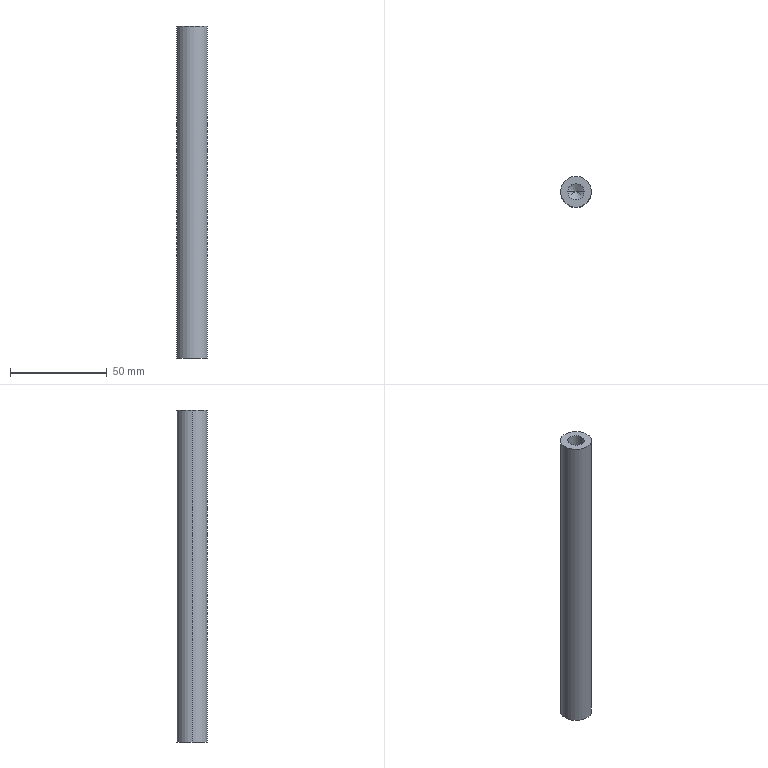Part | STEP file | B1-019 | 1 solid | 12 faces | box 16 x 16 x 172 mm | volume 32897 mm3 | cylinder 6 | cone 4 | plane 2 | commonest cylinder face diameters 8.5 x4 16 x2
STEP:
#1=CARTESIAN_POINT('',(0.,0.,0.));
#2=DIRECTION('',(0.,0.,1.));
#3=DIRECTION('',(1.,0.,0.));
#4=AXIS2_PLACEMENT_3D('',#1,#2,#3);
#5=CARTESIAN_POINT('',(4.25,0.,72.));
#6=VERTEX_POINT('',#5);
#7=CARTESIAN_POINT('',(4.25,0.,86.));
#8=VERTEX_POINT('',#7);
#9=CARTESIAN_POINT('',(4.25,0.,86.));
#10=DIRECTION('',(0.,0.,1.));
#11=VECTOR('',#10,1.);
#12=LINE('',#9,#11);
#13=CARTESIAN_POINT('',(0.,0.,86.));
#14=DIRECTION('',(0.,0.,1.));
#15=DIRECTION('',(1.,0.,0.));
#16=AXIS2_PLACEMENT_3D('',#13,#14,#15);
#17=CYLINDRICAL_SURFACE('',#16,4.25);
#18=CARTESIAN_POINT('',(6.283,0.));
#19=DIRECTION('',(0.,1.));
#20=VECTOR('',#19,1.);
#21=LINE('',#18,#20);
#22=(GEOMETRIC_REPRESENTATION_CONTEXT(2)PARAMETRIC_REPRESENTATION_CONTEXT()REPRESENTATION_CONTEXT('',''));
#23=DEFINITIONAL_REPRESENTATION('',(#21),#22);
#24=PCURVE('',#17,#23);
#25=CARTESIAN_POINT('',(0.,0.,86.));
#26=DIRECTION('',(0.,0.,1.));
#27=DIRECTION('',(1.,0.,0.));
#28=AXIS2_PLACEMENT_3D('',#25,#26,#27);
#29=CYLINDRICAL_SURFACE('',#28,4.25);
#30=CARTESIAN_POINT('',(0.,0.));
#31=DIRECTION('',(0.,1.));
#32=VECTOR('',#31,1.);
#33=LINE('',#30,#32);
#34=(GEOMETRIC_REPRESENTATION_CONTEXT(2)PARAMETRIC_REPRESENTATION_CONTEXT()REPRESENTATION_CONTEXT('',''));
#35=DEFINITIONAL_REPRESENTATION('',(#33),#34);
#36=PCURVE('',#29,#35);
#37=SURFACE_CURVE('',#12,(#24,#36),.PCURVE_S1.);
#38=EDGE_CURVE('',#6,#8,#37,.T.);
#39=ORIENTED_EDGE('',*,*,#38,.T.);
#40=CARTESIAN_POINT('',(-4.25,0.,86.));
#41=VERTEX_POINT('',#40);
#42=CARTESIAN_POINT('',(0.,0.,86.));
#43=DIRECTION('',(0.,0.,1.));
#44=DIRECTION('',(1.,0.,0.));
#45=AXIS2_PLACEMENT_3D('',#42,#43,#44);
#46=CIRCLE('',#45,4.25);
#47=CARTESIAN_POINT('',(0.,0.));
#48=DIRECTION('',(1.,0.));
#49=VECTOR('',#48,1.);
#50=LINE('',#47,#49);
#51=(GEOMETRIC_REPRESENTATION_CONTEXT(2)PARAMETRIC_REPRESENTATION_CONTEXT()REPRESENTATION_CONTEXT('',''));
#52=DEFINITIONAL_REPRESENTATION('',(#50),#51);
#53=PCURVE('',#17,#52);
#54=CARTESIAN_POINT('',(0.,0.,86.));
#55=DIRECTION('',(0.,0.,1.));
#56=DIRECTION('',(1.,0.,0.));
#57=AXIS2_PLACEMENT_3D('',#54,#55,#56);
#58=PLANE('',#57);
#59=CARTESIAN_POINT('',(0.,0.));
#60=DIRECTION('',(1.,0.));
#61=AXIS2_PLACEMENT_2D('',#59,#60);
#62=CIRCLE('',#61,4.25);
#63=(GEOMETRIC_REPRESENTATION_CONTEXT(2)PARAMETRIC_REPRESENTATION_CONTEXT()REPRESENTATION_CONTEXT('',''));
#64=DEFINITIONAL_REPRESENTATION('',(#62),#63);
#65=PCURVE('',#58,#64);
#66=SURFACE_CURVE('',#46,(#53,#65),.PCURVE_S1.);
#67=EDGE_CURVE('',#41,#8,#66,.T.);
#68=ORIENTED_EDGE('',*,*,#67,.F.);
#69=CARTESIAN_POINT('',(-4.25,0.,72.));
#70=VERTEX_POINT('',#69);
#71=CARTESIAN_POINT('',(-4.25,0.,86.));
#72=DIRECTION('',(0.,0.,1.));
#73=VECTOR('',#72,1.);
#74=LINE('',#71,#73);
#75=CARTESIAN_POINT('',(3.142,0.));
#76=DIRECTION('',(0.,1.));
#77=VECTOR('',#76,1.);
#78=LINE('',#75,#77);
#79=(GEOMETRIC_REPRESENTATION_CONTEXT(2)PARAMETRIC_REPRESENTATION_CONTEXT()REPRESENTATION_CONTEXT('',''));
#80=DEFINITIONAL_REPRESENTATION('',(#78),#79);
#81=PCURVE('',#17,#80);
#82=CARTESIAN_POINT('',(3.142,0.));
#83=DIRECTION('',(0.,1.));
#84=VECTOR('',#83,1.);
#85=LINE('',#82,#84);
#86=(GEOMETRIC_REPRESENTATION_CONTEXT(2)PARAMETRIC_REPRESENTATION_CONTEXT()REPRESENTATION_CONTEXT('',''));
#87=DEFINITIONAL_REPRESENTATION('',(#85),#86);
#88=PCURVE('',#29,#87);
#89=SURFACE_CURVE('',#74,(#81,#88),.PCURVE_S1.);
#90=EDGE_CURVE('',#70,#41,#89,.T.);
#91=ORIENTED_EDGE('',*,*,#90,.F.);
#92=CARTESIAN_POINT('',(0.,0.,72.));
#93=DIRECTION('',(0.,0.,1.));
#94=DIRECTION('',(1.,0.,0.));
#95=AXIS2_PLACEMENT_3D('',#92,#93,#94);
#96=CIRCLE('',#95,4.25);
#97=CARTESIAN_POINT('',(0.,-14.));
#98=DIRECTION('',(1.,0.));
#99=VECTOR('',#98,1.);
#100=LINE('',#97,#99);
#101=(GEOMETRIC_REPRESENTATION_CONTEXT(2)PARAMETRIC_REPRESENTATION_CONTEXT()REPRESENTATION_CONTEXT('',''));
#102=DEFINITIONAL_REPRESENTATION('',(#100),#101);
#103=PCURVE('',#17,#102);
#104=CARTESIAN_POINT('',(0.,0.,72.));
#105=DIRECTION('',(0.,0.,1.));
#106=DIRECTION('',(1.,0.,0.));
#107=AXIS2_PLACEMENT_3D('',#104,#105,#106);
#108=CONICAL_SURFACE('',#107,4.25,1.03);
#109=CARTESIAN_POINT('',(0.,0.));
#110=DIRECTION('',(1.,0.));
#111=VECTOR('',#110,1.);
#112=LINE('',#109,#111);
#113=(GEOMETRIC_REPRESENTATION_CONTEXT(2)PARAMETRIC_REPRESENTATION_CONTEXT()REPRESENTATION_CONTEXT('',''));
#114=DEFINITIONAL_REPRESENTATION('',(#112),#113);
#115=PCURVE('',#108,#114);
#116=SURFACE_CURVE('',#96,(#103,#115),.PCURVE_S1.);
#117=EDGE_CURVE('',#70,#6,#116,.T.);
#118=ORIENTED_EDGE('',*,*,#117,.T.);
#119=EDGE_LOOP('',(#39,#68,#91,#118));
#120=FACE_BOUND('',#119,.F.);
#121=ADVANCED_FACE('',(#120),#17,.F.);
#122=ORIENTED_EDGE('',*,*,#117,.F.);
#123=CARTESIAN_POINT('',(0.,0.,69.446));
#124=VERTEX_POINT('',#123);
#125=CARTESIAN_POINT('',(-4.25,0.,72.));
#126=DIRECTION('',(-0.8572,0.,0.515));
#127=VECTOR('',#126,1.);
#128=LINE('',#125,#127);
#129=CARTESIAN_POINT('',(3.142,0.));
#130=DIRECTION('',(0.,1.));
#131=VECTOR('',#130,1.);
#132=LINE('',#129,#131);
#133=(GEOMETRIC_REPRESENTATION_CONTEXT(2)PARAMETRIC_REPRESENTATION_CONTEXT()REPRESENTATION_CONTEXT('',''));
#134=DEFINITIONAL_REPRESENTATION('',(#132),#133);
#135=PCURVE('',#108,#134);
#136=CARTESIAN_POINT('',(0.,0.,72.));
#137=DIRECTION('',(0.,0.,1.));
#138=DIRECTION('',(1.,0.,0.));
#139=AXIS2_PLACEMENT_3D('',#136,#137,#138);
#140=CONICAL_SURFACE('',#139,4.25,1.03);
#141=CARTESIAN_POINT('',(3.142,0.));
#142=DIRECTION('',(0.,1.));
#143=VECTOR('',#142,1.);
#144=LINE('',#141,#143);
#145=(GEOMETRIC_REPRESENTATION_CONTEXT(2)PARAMETRIC_REPRESENTATION_CONTEXT()REPRESENTATION_CONTEXT('',''));
#146=DEFINITIONAL_REPRESENTATION('',(#144),#145);
#147=PCURVE('',#140,#146);
#148=SURFACE_CURVE('',#128,(#135,#147),.PCURVE_S1.);
#149=EDGE_CURVE('',#124,#70,#148,.T.);
#150=ORIENTED_EDGE('',*,*,#149,.F.);
#151=CARTESIAN_POINT('',(4.25,0.,72.));
#152=DIRECTION('',(0.8572,0.,0.515));
#153=VECTOR('',#152,1.);
#154=LINE('',#151,#153);
#155=CARTESIAN_POINT('',(6.283,-2.554));
#156=CARTESIAN_POINT('',(6.283,-2.515));
#157=CARTESIAN_POINT('',(6.283,-2.438));
#158=CARTESIAN_POINT('',(6.283,-2.322));
#159=CARTESIAN_POINT('',(6.283,-2.205));
#160=CARTESIAN_POINT('',(6.283,-2.089));
#161=CARTESIAN_POINT('',(6.283,-1.973));
#162=CARTESIAN_POINT('',(6.283,-1.857));
#163=CARTESIAN_POINT('',(6.283,-1.741));
#164=CARTESIAN_POINT('',(6.283,-1.625));
#165=CARTESIAN_POINT('',(6.283,-1.509));
#166=CARTESIAN_POINT('',(6.283,-1.393));
#167=CARTESIAN_POINT('',(6.283,-1.277));
#168=CARTESIAN_POINT('',(6.283,-1.161));
#169=CARTESIAN_POINT('',(6.283,-1.045));
#170=CARTESIAN_POINT('',(6.283,-0.9286));
#171=CARTESIAN_POINT('',(6.283,-0.8125));
#172=CARTESIAN_POINT('',(6.283,-0.6965));
#173=CARTESIAN_POINT('',(6.283,-0.5804));
#174=CARTESIAN_POINT('',(6.283,-0.4643));
#175=CARTESIAN_POINT('',(6.283,-0.3482));
#176=CARTESIAN_POINT('',(6.283,-0.2322));
#177=CARTESIAN_POINT('',(6.283,-0.1161));
#178=CARTESIAN_POINT('',(6.283,-0.03869));
#179=CARTESIAN_POINT('',(6.283,0.));
#180=B_SPLINE_CURVE_WITH_KNOTS('',3,(#155,#156,#157,#158,#159,#160,#161,#162,#163,#164,#165,#166,#167,#168,#169,#170,#171,#172,#173,#174,#175,#176,#177,#178,#179),.UNSPECIFIED.,.F.,.F.,(4,1,1,1,1,1,1,1,1,1,1,1,1,1,1,1,1,1,1,1,1,1,4),(-4.958,-4.733,-4.507,-4.282,-4.057,-3.831,-3.606,-3.381,-3.155,-2.93,-2.704,-2.479,-2.254,-2.028,-1.803,-1.578,-1.352,-1.127,-0.9015,-0.6761,-0.4507,-0.2254,0.),.QUASI_UNIFORM_KNOTS.);
#181=(GEOMETRIC_REPRESENTATION_CONTEXT(2)PARAMETRIC_REPRESENTATION_CONTEXT()REPRESENTATION_CONTEXT('',''));
#182=DEFINITIONAL_REPRESENTATION('',(#180),#181);
#183=PCURVE('',#108,#182);
#184=CARTESIAN_POINT('',(0.,-2.554));
#185=CARTESIAN_POINT('',(0.,-2.515));
#186=CARTESIAN_POINT('',(0.,-2.438));
#187=CARTESIAN_POINT('',(0.,-2.322));
#188=CARTESIAN_POINT('',(0.,-2.205));
#189=CARTESIAN_POINT('',(0.,-2.089));
#190=CARTESIAN_POINT('',(0.,-1.973));
#191=CARTESIAN_POINT('',(0.,-1.857));
#192=CARTESIAN_POINT('',(0.,-1.741));
#193=CARTESIAN_POINT('',(0.,-1.625));
#194=CARTESIAN_POINT('',(0.,-1.509));
#195=CARTESIAN_POINT('',(0.,-1.393));
#196=CARTESIAN_POINT('',(0.,-1.277));
#197=CARTESIAN_POINT('',(0.,-1.161));
#198=CARTESIAN_POINT('',(0.,-1.045));
#199=CARTESIAN_POINT('',(0.,-0.9286));
#200=CARTESIAN_POINT('',(0.,-0.8125));
#201=CARTESIAN_POINT('',(0.,-0.6965));
#202=CARTESIAN_POINT('',(0.,-0.5804));
#203=CARTESIAN_POINT('',(0.,-0.4643));
#204=CARTESIAN_POINT('',(0.,-0.3482));
#205=CARTESIAN_POINT('',(0.,-0.2322));
#206=CARTESIAN_POINT('',(0.,-0.1161));
#207=CARTESIAN_POINT('',(0.,-0.03869));
#208=CARTESIAN_POINT('',(0.,0.));
#209=B_SPLINE_CURVE_WITH_KNOTS('',3,(#184,#185,#186,#187,#188,#189,#190,#191,#192,#193,#194,#195,#196,#197,#198,#199,#200,#201,#202,#203,#204,#205,#206,#207,#208),.UNSPECIFIED.,.F.,.F.,(4,1,1,1,1,1,1,1,1,1,1,1,1,1,1,1,1,1,1,1,1,1,4),(-4.958,-4.733,-4.507,-4.282,-4.057,-3.831,-3.606,-3.381,-3.155,-2.93,-2.704,-2.479,-2.254,-2.028,-1.803,-1.578,-1.352,-1.127,-0.9015,-0.6761,-0.4507,-0.2254,0.),.QUASI_UNIFORM_KNOTS.);
#210=(GEOMETRIC_REPRESENTATION_CONTEXT(2)PARAMETRIC_REPRESENTATION_CONTEXT()REPRESENTATION_CONTEXT('',''));
#211=DEFINITIONAL_REPRESENTATION('',(#209),#210);
#212=PCURVE('',#140,#211);
#213=SURFACE_CURVE('',#154,(#183,#212),.PCURVE_S1.);
#214=EDGE_CURVE('',#124,#6,#213,.T.);
#215=ORIENTED_EDGE('',*,*,#214,.T.);
#216=EDGE_LOOP('',(#122,#150,#215));
#217=FACE_BOUND('',#216,.F.);
#218=ADVANCED_FACE('',(#217),#108,.F.);
#219=CARTESIAN_POINT('',(-4.25,0.,-72.));
#220=VERTEX_POINT('',#219);
#221=CARTESIAN_POINT('',(-4.25,0.,-86.));
#222=VERTEX_POINT('',#221);
#223=CARTESIAN_POINT('',(-4.25,0.,-86.));
#224=DIRECTION('',(0.,0.,-1.));
#225=VECTOR('',#224,1.);
#226=LINE('',#223,#225);
#227=CARTESIAN_POINT('',(0.,0.,-86.));
#228=DIRECTION('',(0.,0.,-1.));
#229=DIRECTION('',(-1.,0.,0.));
#230=AXIS2_PLACEMENT_3D('',#227,#228,#229);
#231=CYLINDRICAL_SURFACE('',#230,4.25);
#232=CARTESIAN_POINT('',(6.283,0.));
#233=DIRECTION('',(0.,1.));
#234=VECTOR('',#233,1.);
#235=LINE('',#232,#234);
#236=(GEOMETRIC_REPRESENTATION_CONTEXT(2)PARAMETRIC_REPRESENTATION_CONTEXT()REPRESENTATION_CONTEXT('',''));
#237=DEFINITIONAL_REPRESENTATION('',(#235),#236);
#238=PCURVE('',#231,#237);
#239=CARTESIAN_POINT('',(0.,0.,-86.));
#240=DIRECTION('',(0.,0.,-1.));
#241=DIRECTION('',(-1.,0.,0.));
#242=AXIS2_PLACEMENT_3D('',#239,#240,#241);
#243=CYLINDRICAL_SURFACE('',#242,4.25);
#244=CARTESIAN_POINT('',(0.,0.));
#245=DIRECTION('',(0.,1.));
#246=VECTOR('',#245,1.);
#247=LINE('',#244,#246);
#248=(GEOMETRIC_REPRESENTATION_CONTEXT(2)PARAMETRIC_REPRESENTATION_CONTEXT()REPRESENTATION_CONTEXT('',''));
#249=DEFINITIONAL_REPRESENTATION('',(#247),#248);
#250=PCURVE('',#243,#249);
#251=SURFACE_CURVE('',#226,(#238,#250),.PCURVE_S1.);
#252=EDGE_CURVE('',#220,#222,#251,.T.);
#253=ORIENTED_EDGE('',*,*,#252,.T.);
#254=CARTESIAN_POINT('',(4.25,0.,-86.));
#255=VERTEX_POINT('',#254);
#256=CARTESIAN_POINT('',(0.,0.,-86.));
#257=DIRECTION('',(0.,0.,-1.));
#258=DIRECTION('',(-1.,0.,0.));
#259=AXIS2_PLACEMENT_3D('',#256,#257,#258);
#260=CIRCLE('',#259,4.25);
#261=CARTESIAN_POINT('',(0.,0.));
#262=DIRECTION('',(1.,0.));
#263=VECTOR('',#262,1.);
#264=LINE('',#261,#263);
#265=(GEOMETRIC_REPRESENTATION_CONTEXT(2)PARAMETRIC_REPRESENTATION_CONTEXT()REPRESENTATION_CONTEXT('',''));
#266=DEFINITIONAL_REPRESENTATION('',(#264),#265);
#267=PCURVE('',#231,#266);
#268=CARTESIAN_POINT('',(0.,0.,-86.));
#269=DIRECTION('',(0.,0.,1.));
#270=DIRECTION('',(1.,0.,0.));
#271=AXIS2_PLACEMENT_3D('',#268,#269,#270);
#272=PLANE('',#271);
#273=CARTESIAN_POINT('',(-4.25,0.));
#274=CARTESIAN_POINT('',(-4.25,7.361));
#275=CARTESIAN_POINT('',(2.125,3.681));
#276=CARTESIAN_POINT('',(8.5,0.));
#277=CARTESIAN_POINT('',(2.125,-3.681));
#278=CARTESIAN_POINT('',(-4.25,-7.361));
#279=CARTESIAN_POINT('',(-4.25,0.));
#280=(BOUNDED_CURVE()B_SPLINE_CURVE(2,(#273,#274,#275,#276,#277,#278,#279),.UNSPECIFIED.,.T.,.F.)B_SPLINE_CURVE_WITH_KNOTS((1,2,2,2,2,1),(-2.094,0.,2.094,4.189,6.283,8.378),.UNSPECIFIED.)CURVE()GEOMETRIC_REPRESENTATION_ITEM()RATIONAL_B_SPLINE_CURVE((1.,0.5,1.,0.5,1.,0.5,1.))REPRESENTATION_ITEM(''));
#281=(GEOMETRIC_REPRESENTATION_CONTEXT(2)PARAMETRIC_REPRESENTATION_CONTEXT()REPRESENTATION_CONTEXT('',''));
#282=DEFINITIONAL_REPRESENTATION('',(#280),#281);
#283=PCURVE('',#272,#282);
#284=SURFACE_CURVE('',#260,(#267,#283),.PCURVE_S1.);
#285=EDGE_CURVE('',#255,#222,#284,.T.);
#286=ORIENTED_EDGE('',*,*,#285,.F.);
#287=CARTESIAN_POINT('',(4.25,0.,-72.));
#288=VERTEX_POINT('',#287);
#289=CARTESIAN_POINT('',(4.25,0.,-86.));
#290=DIRECTION('',(0.,0.,-1.));
#291=VECTOR('',#290,1.);
#292=LINE('',#289,#291);
#293=CARTESIAN_POINT('',(3.142,0.));
#294=DIRECTION('',(0.,1.));
#295=VECTOR('',#294,1.);
#296=LINE('',#293,#295);
#297=(GEOMETRIC_REPRESENTATION_CONTEXT(2)PARAMETRIC_REPRESENTATION_CONTEXT()REPRESENTATION_CONTEXT('',''));
#298=DEFINITIONAL_REPRESENTATION('',(#296),#297);
#299=PCURVE('',#231,#298);
#300=CARTESIAN_POINT('',(3.142,0.));
#301=DIRECTION('',(0.,1.));
#302=VECTOR('',#301,1.);
#303=LINE('',#300,#302);
#304=(GEOMETRIC_REPRESENTATION_CONTEXT(2)PARAMETRIC_REPRESENTATION_CONTEXT()REPRESENTATION_CONTEXT('',''));
#305=DEFINITIONAL_REPRESENTATION('',(#303),#304);
#306=PCURVE('',#243,#305);
#307=SURFACE_CURVE('',#292,(#299,#306),.PCURVE_S1.);
#308=EDGE_CURVE('',#288,#255,#307,.T.);
#309=ORIENTED_EDGE('',*,*,#308,.F.);
#310=CARTESIAN_POINT('',(0.,0.,-72.));
#311=DIRECTION('',(0.,0.,-1.));
#312=DIRECTION('',(-1.,0.,0.));
#313=AXIS2_PLACEMENT_3D('',#310,#311,#312);
#314=CIRCLE('',#313,4.25);
#315=CARTESIAN_POINT('',(0.,-14.));
#316=DIRECTION('',(1.,0.));
#317=VECTOR('',#316,1.);
#318=LINE('',#315,#317);
#319=(GEOMETRIC_REPRESENTATION_CONTEXT(2)PARAMETRIC_REPRESENTATION_CONTEXT()REPRESENTATION_CONTEXT('',''));
#320=DEFINITIONAL_REPRESENTATION('',(#318),#319);
#321=PCURVE('',#231,#320);
#322=CARTESIAN_POINT('',(0.,0.,-72.));
#323=DIRECTION('',(0.,0.,-1.));
#324=DIRECTION('',(-1.,0.,0.));
#325=AXIS2_PLACEMENT_3D('',#322,#323,#324);
#326=CONICAL_SURFACE('',#325,4.25,1.03);
#327=CARTESIAN_POINT('',(0.,0.));
#328=DIRECTION('',(1.,0.));
#329=VECTOR('',#328,1.);
#330=LINE('',#327,#329);
#331=(GEOMETRIC_REPRESENTATION_CONTEXT(2)PARAMETRIC_REPRESENTATION_CONTEXT()REPRESENTATION_CONTEXT('',''));
#332=DEFINITIONAL_REPRESENTATION('',(#330),#331);
#333=PCURVE('',#326,#332);
#334=SURFACE_CURVE('',#314,(#321,#333),.PCURVE_S1.);
#335=EDGE_CURVE('',#288,#220,#334,.T.);
#336=ORIENTED_EDGE('',*,*,#335,.T.);
#337=EDGE_LOOP('',(#253,#286,#309,#336));
#338=FACE_BOUND('',#337,.F.);
#339=ADVANCED_FACE('',(#338),#231,.F.);
#340=ORIENTED_EDGE('',*,*,#335,.F.);
#341=CARTESIAN_POINT('',(0.,0.,-69.446));
#342=VERTEX_POINT('',#341);
#343=CARTESIAN_POINT('',(4.25,0.,-72.));
#344=DIRECTION('',(0.8572,0.,-0.515));
#345=VECTOR('',#344,1.);
#346=LINE('',#343,#345);
#347=CARTESIAN_POINT('',(3.142,-2.554));
#348=CARTESIAN_POINT('',(3.142,-2.515));
#349=CARTESIAN_POINT('',(3.142,-2.438));
#350=CARTESIAN_POINT('',(3.142,-2.322));
#351=CARTESIAN_POINT('',(3.142,-2.205));
#352=CARTESIAN_POINT('',(3.142,-2.089));
#353=CARTESIAN_POINT('',(3.142,-1.973));
#354=CARTESIAN_POINT('',(3.142,-1.857));
#355=CARTESIAN_POINT('',(3.142,-1.741));
#356=CARTESIAN_POINT('',(3.142,-1.625));
#357=CARTESIAN_POINT('',(3.142,-1.509));
#358=CARTESIAN_POINT('',(3.142,-1.393));
#359=CARTESIAN_POINT('',(3.142,-1.277));
#360=CARTESIAN_POINT('',(3.142,-1.161));
#361=CARTESIAN_POINT('',(3.142,-1.045));
#362=CARTESIAN_POINT('',(3.142,-0.9286));
#363=CARTESIAN_POINT('',(3.142,-0.8125));
#364=CARTESIAN_POINT('',(3.142,-0.6965));
#365=CARTESIAN_POINT('',(3.142,-0.5804));
#366=CARTESIAN_POINT('',(3.142,-0.4643));
#367=CARTESIAN_POINT('',(3.142,-0.3482));
#368=CARTESIAN_POINT('',(3.142,-0.2322));
#369=CARTESIAN_POINT('',(3.142,-0.1161));
#370=CARTESIAN_POINT('',(3.142,-0.03869));
#371=CARTESIAN_POINT('',(3.142,0.));
#372=B_SPLINE_CURVE_WITH_KNOTS('',3,(#347,#348,#349,#350,#351,#352,#353,#354,#355,#356,#357,#358,#359,#360,#361,#362,#363,#364,#365,#366,#367,#368,#369,#370,#371),.UNSPECIFIED.,.F.,.F.,(4,1,1,1,1,1,1,1,1,1,1,1,1,1,1,1,1,1,1,1,1,1,4),(-4.958,-4.733,-4.507,-4.282,-4.057,-3.831,-3.606,-3.381,-3.155,-2.93,-2.704,-2.479,-2.254,-2.028,-1.803,-1.578,-1.352,-1.127,-0.9015,-0.6761,-0.4507,-0.2254,0.),.QUASI_UNIFORM_KNOTS.);
#373=(GEOMETRIC_REPRESENTATION_CONTEXT(2)PARAMETRIC_REPRESENTATION_CONTEXT()REPRESENTATION_CONTEXT('',''));
#374=DEFINITIONAL_REPRESENTATION('',(#372),#373);
#375=PCURVE('',#326,#374);
#376=CARTESIAN_POINT('',(0.,0.,-72.));
#377=DIRECTION('',(0.,0.,-1.));
#378=DIRECTION('',(-1.,0.,0.));
#379=AXIS2_PLACEMENT_3D('',#376,#377,#378);
#380=CONICAL_SURFACE('',#379,4.25,1.03);
#381=CARTESIAN_POINT('',(3.142,-2.554));
#382=CARTESIAN_POINT('',(3.142,-2.515));
#383=CARTESIAN_POINT('',(3.142,-2.438));
#384=CARTESIAN_POINT('',(3.142,-2.322));
#385=CARTESIAN_POINT('',(3.142,-2.205));
#386=CARTESIAN_POINT('',(3.142,-2.089));
#387=CARTESIAN_POINT('',(3.142,-1.973));
#388=CARTESIAN_POINT('',(3.142,-1.857));
#389=CARTESIAN_POINT('',(3.142,-1.741));
#390=CARTESIAN_POINT('',(3.142,-1.625));
#391=CARTESIAN_POINT('',(3.142,-1.509));
#392=CARTESIAN_POINT('',(3.142,-1.393));
#393=CARTESIAN_POINT('',(3.142,-1.277));
#394=CARTESIAN_POINT('',(3.142,-1.161));
#395=CARTESIAN_POINT('',(3.142,-1.045));
#396=CARTESIAN_POINT('',(3.142,-0.9286));
#397=CARTESIAN_POINT('',(3.142,-0.8125));
#398=CARTESIAN_POINT('',(3.142,-0.6965));
#399=CARTESIAN_POINT('',(3.142,-0.5804));
#400=CARTESIAN_POINT('',(3.142,-0.4643));
#401=CARTESIAN_POINT('',(3.142,-0.3482));
#402=CARTESIAN_POINT('',(3.142,-0.2322));
#403=CARTESIAN_POINT('',(3.142,-0.1161));
#404=CARTESIAN_POINT('',(3.142,-0.03869));
#405=CARTESIAN_POINT('',(3.142,0.));
#406=B_SPLINE_CURVE_WITH_KNOTS('',3,(#381,#382,#383,#384,#385,#386,#387,#388,#389,#390,#391,#392,#393,#394,#395,#396,#397,#398,#399,#400,#401,#402,#403,#404,#405),.UNSPECIFIED.,.F.,.F.,(4,1,1,1,1,1,1,1,1,1,1,1,1,1,1,1,1,1,1,1,1,1,4),(-4.958,-4.733,-4.507,-4.282,-4.057,-3.831,-3.606,-3.381,-3.155,-2.93,-2.704,-2.479,-2.254,-2.028,-1.803,-1.578,-1.352,-1.127,-0.9015,-0.6761,-0.4507,-0.2254,0.),.QUASI_UNIFORM_KNOTS.);
#407=(GEOMETRIC_REPRESENTATION_CONTEXT(2)PARAMETRIC_REPRESENTATION_CONTEXT()REPRESENTATION_CONTEXT('',''));
#408=DEFINITIONAL_REPRESENTATION('',(#406),#407);
#409=PCURVE('',#380,#408);
#410=SURFACE_CURVE('',#346,(#375,#409),.PCURVE_S1.);
#411=EDGE_CURVE('',#342,#288,#410,.T.);
#412=ORIENTED_EDGE('',*,*,#411,.F.);
#413=CARTESIAN_POINT('',(-4.25,0.,-72.));
#414=DIRECTION('',(-0.8572,0.,-0.515));
#415=VECTOR('',#414,1.);
#416=LINE('',#413,#415);
#417=CARTESIAN_POINT('',(6.283,0.));
#418=DIRECTION('',(0.,1.));
#419=VECTOR('',#418,1.);
#420=LINE('',#417,#419);
#421=(GEOMETRIC_REPRESENTATION_CONTEXT(2)PARAMETRIC_REPRESENTATION_CONTEXT()REPRESENTATION_CONTEXT('',''));
#422=DEFINITIONAL_REPRESENTATION('',(#420),#421);
#423=PCURVE('',#326,#422);
#424=CARTESIAN_POINT('',(0.,0.));
#425=DIRECTION('',(0.,1.));
#426=VECTOR('',#425,1.);
#427=LINE('',#424,#426);
#428=(GEOMETRIC_REPRESENTATION_CONTEXT(2)PARAMETRIC_REPRESENTATION_CONTEXT()REPRESENTATION_CONTEXT('',''));
#429=DEFINITIONAL_REPRESENTATION('',(#427),#428);
#430=PCURVE('',#380,#429);
#431=SURFACE_CURVE('',#416,(#423,#430),.PCURVE_S1.);
#432=EDGE_CURVE('',#342,#220,#431,.T.);
#433=ORIENTED_EDGE('',*,*,#432,.T.);
#434=EDGE_LOOP('',(#340,#412,#433));
#435=FACE_BOUND('',#434,.F.);
#436=ADVANCED_FACE('',(#435),#326,.F.);
#437=CARTESIAN_POINT('',(8.,0.,86.));
#438=VERTEX_POINT('',#437);
#439=CARTESIAN_POINT('',(-8.,0.,86.));
#440=VERTEX_POINT('',#439);
#441=CARTESIAN_POINT('',(0.,0.,86.));
#442=DIRECTION('',(0.,0.,1.));
#443=DIRECTION('',(1.,0.,0.));
#444=AXIS2_PLACEMENT_3D('',#441,#442,#443);
#445=CIRCLE('',#444,8.);
#446=CARTESIAN_POINT('',(0.,0.,86.));
#447=DIRECTION('',(0.,0.,-1.));
#448=DIRECTION('',(-1.,0.,0.));
#449=AXIS2_PLACEMENT_3D('',#446,#447,#448);
#450=CYLINDRICAL_SURFACE('',#449,8.);
#451=CARTESIAN_POINT('',(3.142,0.));
#452=DIRECTION('',(-1.,0.));
#453=VECTOR('',#452,1.);
#454=LINE('',#451,#453);
#455=(GEOMETRIC_REPRESENTATION_CONTEXT(2)PARAMETRIC_REPRESENTATION_CONTEXT()REPRESENTATION_CONTEXT('',''));
#456=DEFINITIONAL_REPRESENTATION('',(#454),#455);
#457=PCURVE('',#450,#456);
#458=CARTESIAN_POINT('',(0.,0.));
#459=DIRECTION('',(1.,0.));
#460=AXIS2_PLACEMENT_2D('',#458,#459);
#461=CIRCLE('',#460,8.);
#462=(GEOMETRIC_REPRESENTATION_CONTEXT(2)PARAMETRIC_REPRESENTATION_CONTEXT()REPRESENTATION_CONTEXT('',''));
#463=DEFINITIONAL_REPRESENTATION('',(#461),#462);
#464=PCURVE('',#58,#463);
#465=SURFACE_CURVE('',#445,(#457,#464),.PCURVE_S1.);
#466=EDGE_CURVE('',#438,#440,#465,.T.);
#467=ORIENTED_EDGE('',*,*,#466,.F.);
#468=CARTESIAN_POINT('',(8.,0.,-86.));
#469=VERTEX_POINT('',#468);
#470=CARTESIAN_POINT('',(8.,0.,86.));
#471=DIRECTION('',(0.,0.,-1.));
#472=VECTOR('',#471,1.);
#473=LINE('',#470,#472);
#474=CARTESIAN_POINT('',(3.142,0.));
#475=DIRECTION('',(0.,1.));
#476=VECTOR('',#475,1.);
#477=LINE('',#474,#476);
#478=(GEOMETRIC_REPRESENTATION_CONTEXT(2)PARAMETRIC_REPRESENTATION_CONTEXT()REPRESENTATION_CONTEXT('',''));
#479=DEFINITIONAL_REPRESENTATION('',(#477),#478);
#480=PCURVE('',#450,#479);
#481=CARTESIAN_POINT('',(0.,0.,86.));
#482=DIRECTION('',(0.,0.,-1.));
#483=DIRECTION('',(-1.,0.,0.));
#484=AXIS2_PLACEMENT_3D('',#481,#482,#483);
#485=CYLINDRICAL_SURFACE('',#484,8.);
#486=CARTESIAN_POINT('',(3.142,0.));
#487=DIRECTION('',(0.,1.));
#488=VECTOR('',#487,1.);
#489=LINE('',#486,#488);
#490=(GEOMETRIC_REPRESENTATION_CONTEXT(2)PARAMETRIC_REPRESENTATION_CONTEXT()REPRESENTATION_CONTEXT('',''));
#491=DEFINITIONAL_REPRESENTATION('',(#489),#490);
#492=PCURVE('',#485,#491);
#493=SURFACE_CURVE('',#473,(#480,#492),.PCURVE_S1.);
#494=EDGE_CURVE('',#438,#469,#493,.T.);
#495=ORIENTED_EDGE('',*,*,#494,.T.);
#496=CARTESIAN_POINT('',(-8.,0.,-86.));
#497=VERTEX_POINT('',#496);
#498=CARTESIAN_POINT('',(0.,0.,-86.));
#499=DIRECTION('',(0.,0.,1.));
#500=DIRECTION('',(1.,0.,0.));
#501=AXIS2_PLACEMENT_3D('',#498,#499,#500);
#502=CIRCLE('',#501,8.);
#503=CARTESIAN_POINT('',(3.142,172.));
#504=DIRECTION('',(-1.,0.));
#505=VECTOR('',#504,1.);
#506=LINE('',#503,#505);
#507=(GEOMETRIC_REPRESENTATION_CONTEXT(2)PARAMETRIC_REPRESENTATION_CONTEXT()REPRESENTATION_CONTEXT('',''));
#508=DEFINITIONAL_REPRESENTATION('',(#506),#507);
#509=PCURVE('',#450,#508);
#510=CARTESIAN_POINT('',(0.,0.));
#511=DIRECTION('',(1.,0.));
#512=AXIS2_PLACEMENT_2D('',#510,#511);
#513=CIRCLE('',#512,8.);
#514=(GEOMETRIC_REPRESENTATION_CONTEXT(2)PARAMETRIC_REPRESENTATION_CONTEXT()REPRESENTATION_CONTEXT('',''));
#515=DEFINITIONAL_REPRESENTATION('',(#513),#514);
#516=PCURVE('',#272,#515);
#517=SURFACE_CURVE('',#502,(#509,#516),.PCURVE_S1.);
#518=EDGE_CURVE('',#469,#497,#517,.T.);
#519=ORIENTED_EDGE('',*,*,#518,.T.);
#520=CARTESIAN_POINT('',(-8.,0.,86.));
#521=DIRECTION('',(0.,0.,-1.));
#522=VECTOR('',#521,1.);
#523=LINE('',#520,#522);
#524=CARTESIAN_POINT('',(0.,0.));
#525=DIRECTION('',(0.,1.));
#526=VECTOR('',#525,1.);
#527=LINE('',#524,#526);
#528=(GEOMETRIC_REPRESENTATION_CONTEXT(2)PARAMETRIC_REPRESENTATION_CONTEXT()REPRESENTATION_CONTEXT('',''));
#529=DEFINITIONAL_REPRESENTATION('',(#527),#528);
#530=PCURVE('',#450,#529);
#531=CARTESIAN_POINT('',(6.283,0.));
#532=DIRECTION('',(0.,1.));
#533=VECTOR('',#532,1.);
#534=LINE('',#531,#533);
#535=(GEOMETRIC_REPRESENTATION_CONTEXT(2)PARAMETRIC_REPRESENTATION_CONTEXT()REPRESENTATION_CONTEXT('',''));
#536=DEFINITIONAL_REPRESENTATION('',(#534),#535);
#537=PCURVE('',#485,#536);
#538=SURFACE_CURVE('',#523,(#530,#537),.PCURVE_S1.);
#539=EDGE_CURVE('',#440,#497,#538,.T.);
#540=ORIENTED_EDGE('',*,*,#539,.F.);
#541=EDGE_LOOP('',(#467,#495,#519,#540));
#542=FACE_BOUND('',#541,.T.);
#543=ADVANCED_FACE('',(#542),#450,.T.);
#544=ORIENTED_EDGE('',*,*,#494,.F.);
#545=CARTESIAN_POINT('',(0.,0.,86.));
#546=DIRECTION('',(0.,0.,1.));
#547=DIRECTION('',(1.,0.,0.));
#548=AXIS2_PLACEMENT_3D('',#545,#546,#547);
#549=CIRCLE('',#548,8.);
#550=CARTESIAN_POINT('',(9.425,0.));
#551=DIRECTION('',(-1.,0.));
#552=VECTOR('',#551,1.);
#553=LINE('',#550,#552);
#554=(GEOMETRIC_REPRESENTATION_CONTEXT(2)PARAMETRIC_REPRESENTATION_CONTEXT()REPRESENTATION_CONTEXT('',''));
#555=DEFINITIONAL_REPRESENTATION('',(#553),#554);
#556=PCURVE('',#485,#555);
#557=CARTESIAN_POINT('',(0.,0.));
#558=DIRECTION('',(1.,0.));
#559=AXIS2_PLACEMENT_2D('',#557,#558);
#560=CIRCLE('',#559,8.);
#561=(GEOMETRIC_REPRESENTATION_CONTEXT(2)PARAMETRIC_REPRESENTATION_CONTEXT()REPRESENTATION_CONTEXT('',''));
#562=DEFINITIONAL_REPRESENTATION('',(#560),#561);
#563=PCURVE('',#58,#562);
#564=SURFACE_CURVE('',#549,(#556,#563),.PCURVE_S1.);
#565=EDGE_CURVE('',#440,#438,#564,.T.);
#566=ORIENTED_EDGE('',*,*,#565,.F.);
#567=ORIENTED_EDGE('',*,*,#539,.T.);
#568=CARTESIAN_POINT('',(0.,0.,-86.));
#569=DIRECTION('',(0.,0.,1.));
#570=DIRECTION('',(1.,0.,0.));
#571=AXIS2_PLACEMENT_3D('',#568,#569,#570);
#572=CIRCLE('',#571,8.);
#573=CARTESIAN_POINT('',(9.425,172.));
#574=DIRECTION('',(-1.,0.));
#575=VECTOR('',#574,1.);
#576=LINE('',#573,#575);
#577=(GEOMETRIC_REPRESENTATION_CONTEXT(2)PARAMETRIC_REPRESENTATION_CONTEXT()REPRESENTATION_CONTEXT('',''));
#578=DEFINITIONAL_REPRESENTATION('',(#576),#577);
#579=PCURVE('',#485,#578);
#580=CARTESIAN_POINT('',(0.,0.));
#581=DIRECTION('',(1.,0.));
#582=AXIS2_PLACEMENT_2D('',#580,#581);
#583=CIRCLE('',#582,8.);
#584=(GEOMETRIC_REPRESENTATION_CONTEXT(2)PARAMETRIC_REPRESENTATION_CONTEXT()REPRESENTATION_CONTEXT('',''));
#585=DEFINITIONAL_REPRESENTATION('',(#583),#584);
#586=PCURVE('',#272,#585);
#587=SURFACE_CURVE('',#572,(#579,#586),.PCURVE_S1.);
#588=EDGE_CURVE('',#497,#469,#587,.T.);
#589=ORIENTED_EDGE('',*,*,#588,.T.);
#590=EDGE_LOOP('',(#544,#566,#567,#589));
#591=FACE_BOUND('',#590,.T.);
#592=ADVANCED_FACE('',(#591),#485,.T.);
#593=CARTESIAN_POINT('',(0.,0.,86.));
#594=DIRECTION('',(0.,0.,1.));
#595=DIRECTION('',(1.,0.,0.));
#596=AXIS2_PLACEMENT_3D('',#593,#594,#595);
#597=CIRCLE('',#596,4.25);
#598=CARTESIAN_POINT('',(0.,0.));
#599=DIRECTION('',(1.,0.));
#600=AXIS2_PLACEMENT_2D('',#598,#599);
#601=CIRCLE('',#600,4.25);
#602=(GEOMETRIC_REPRESENTATION_CONTEXT(2)PARAMETRIC_REPRESENTATION_CONTEXT()REPRESENTATION_CONTEXT('',''));
#603=DEFINITIONAL_REPRESENTATION('',(#601),#602);
#604=PCURVE('',#58,#603);
#605=CARTESIAN_POINT('',(0.,0.));
#606=DIRECTION('',(1.,0.));
#607=VECTOR('',#606,1.);
#608=LINE('',#605,#607);
#609=(GEOMETRIC_REPRESENTATION_CONTEXT(2)PARAMETRIC_REPRESENTATION_CONTEXT()REPRESENTATION_CONTEXT('',''));
#610=DEFINITIONAL_REPRESENTATION('',(#608),#609);
#611=PCURVE('',#29,#610);
#612=SURFACE_CURVE('',#597,(#604,#611),.PCURVE_S1.);
#613=EDGE_CURVE('',#8,#41,#612,.T.);
#614=ORIENTED_EDGE('',*,*,#613,.F.);
#615=ORIENTED_EDGE('',*,*,#67,.F.);
#616=EDGE_LOOP('',(#614,#615));
#617=FACE_BOUND('',#616,.T.);
#618=ORIENTED_EDGE('',*,*,#565,.T.);
#619=ORIENTED_EDGE('',*,*,#466,.T.);
#620=EDGE_LOOP('',(#618,#619));
#621=FACE_BOUND('',#620,.T.);
#622=ADVANCED_FACE('',(#617,#621),#58,.T.);
#623=CARTESIAN_POINT('',(0.,0.,-86.));
#624=DIRECTION('',(0.,0.,-1.));
#625=DIRECTION('',(-1.,0.,0.));
#626=AXIS2_PLACEMENT_3D('',#623,#624,#625);
#627=CIRCLE('',#626,4.25);
#628=CARTESIAN_POINT('',(-4.25,0.));
#629=CARTESIAN_POINT('',(-4.25,7.361));
#630=CARTESIAN_POINT('',(2.125,3.681));
#631=CARTESIAN_POINT('',(8.5,0.));
#632=CARTESIAN_POINT('',(2.125,-3.681));
#633=CARTESIAN_POINT('',(-4.25,-7.361));
#634=CARTESIAN_POINT('',(-4.25,0.));
#635=(BOUNDED_CURVE()B_SPLINE_CURVE(2,(#628,#629,#630,#631,#632,#633,#634),.UNSPECIFIED.,.T.,.F.)B_SPLINE_CURVE_WITH_KNOTS((1,2,2,2,2,1),(-2.094,0.,2.094,4.189,6.283,8.378),.UNSPECIFIED.)CURVE()GEOMETRIC_REPRESENTATION_ITEM()RATIONAL_B_SPLINE_CURVE((1.,0.5,1.,0.5,1.,0.5,1.))REPRESENTATION_ITEM(''));
#636=(GEOMETRIC_REPRESENTATION_CONTEXT(2)PARAMETRIC_REPRESENTATION_CONTEXT()REPRESENTATION_CONTEXT('',''));
#637=DEFINITIONAL_REPRESENTATION('',(#635),#636);
#638=PCURVE('',#272,#637);
#639=CARTESIAN_POINT('',(0.,0.));
#640=DIRECTION('',(1.,0.));
#641=VECTOR('',#640,1.);
#642=LINE('',#639,#641);
#643=(GEOMETRIC_REPRESENTATION_CONTEXT(2)PARAMETRIC_REPRESENTATION_CONTEXT()REPRESENTATION_CONTEXT('',''));
#644=DEFINITIONAL_REPRESENTATION('',(#642),#643);
#645=PCURVE('',#243,#644);
#646=SURFACE_CURVE('',#627,(#638,#645),.PCURVE_S1.);
#647=EDGE_CURVE('',#222,#255,#646,.T.);
#648=ORIENTED_EDGE('',*,*,#647,.F.);
#649=ORIENTED_EDGE('',*,*,#285,.F.);
#650=EDGE_LOOP('',(#648,#649));
#651=FACE_BOUND('',#650,.T.);
#652=ORIENTED_EDGE('',*,*,#588,.F.);
#653=ORIENTED_EDGE('',*,*,#518,.F.);
#654=EDGE_LOOP('',(#652,#653));
#655=FACE_BOUND('',#654,.T.);
#656=ADVANCED_FACE('',(#651,#655),#272,.F.);
#657=CARTESIAN_POINT('',(0.,0.,-72.));
#658=DIRECTION('',(0.,0.,-1.));
#659=DIRECTION('',(-1.,0.,0.));
#660=AXIS2_PLACEMENT_3D('',#657,#658,#659);
#661=CIRCLE('',#660,4.25);
#662=CARTESIAN_POINT('',(0.,0.));
#663=DIRECTION('',(1.,0.));
#664=VECTOR('',#663,1.);
#665=LINE('',#662,#664);
#666=(GEOMETRIC_REPRESENTATION_CONTEXT(2)PARAMETRIC_REPRESENTATION_CONTEXT()REPRESENTATION_CONTEXT('',''));
#667=DEFINITIONAL_REPRESENTATION('',(#665),#666);
#668=PCURVE('',#380,#667);
#669=CARTESIAN_POINT('',(0.,-14.));
#670=DIRECTION('',(1.,0.));
#671=VECTOR('',#670,1.);
#672=LINE('',#669,#671);
#673=(GEOMETRIC_REPRESENTATION_CONTEXT(2)PARAMETRIC_REPRESENTATION_CONTEXT()REPRESENTATION_CONTEXT('',''));
#674=DEFINITIONAL_REPRESENTATION('',(#672),#673);
#675=PCURVE('',#243,#674);
#676=SURFACE_CURVE('',#661,(#668,#675),.PCURVE_S1.);
#677=EDGE_CURVE('',#220,#288,#676,.T.);
#678=ORIENTED_EDGE('',*,*,#677,.F.);
#679=ORIENTED_EDGE('',*,*,#432,.F.);
#680=ORIENTED_EDGE('',*,*,#411,.T.);
#681=EDGE_LOOP('',(#678,#679,#680));
#682=FACE_BOUND('',#681,.F.);
#683=ADVANCED_FACE('',(#682),#380,.F.);
#684=ORIENTED_EDGE('',*,*,#647,.F.);
#685=ORIENTED_EDGE('',*,*,#252,.F.);
#686=ORIENTED_EDGE('',*,*,#677,.T.);
#687=ORIENTED_EDGE('',*,*,#308,.T.);
#688=EDGE_LOOP('',(#684,#685,#686,#687));
#689=FACE_BOUND('',#688,.F.);
#690=ADVANCED_FACE('',(#689),#243,.F.);
#691=CARTESIAN_POINT('',(0.,0.,72.));
#692=DIRECTION('',(0.,0.,1.));
#693=DIRECTION('',(1.,0.,0.));
#694=AXIS2_PLACEMENT_3D('',#691,#692,#693);
#695=CIRCLE('',#694,4.25);
#696=CARTESIAN_POINT('',(0.,0.));
#697=DIRECTION('',(1.,0.));
#698=VECTOR('',#697,1.);
#699=LINE('',#696,#698);
#700=(GEOMETRIC_REPRESENTATION_CONTEXT(2)PARAMETRIC_REPRESENTATION_CONTEXT()REPRESENTATION_CONTEXT('',''));
#701=DEFINITIONAL_REPRESENTATION('',(#699),#700);
#702=PCURVE('',#140,#701);
#703=CARTESIAN_POINT('',(0.,-14.));
#704=DIRECTION('',(1.,0.));
#705=VECTOR('',#704,1.);
#706=LINE('',#703,#705);
#707=(GEOMETRIC_REPRESENTATION_CONTEXT(2)PARAMETRIC_REPRESENTATION_CONTEXT()REPRESENTATION_CONTEXT('',''));
#708=DEFINITIONAL_REPRESENTATION('',(#706),#707);
#709=PCURVE('',#29,#708);
#710=SURFACE_CURVE('',#695,(#702,#709),.PCURVE_S1.);
#711=EDGE_CURVE('',#6,#70,#710,.T.);
#712=ORIENTED_EDGE('',*,*,#711,.F.);
#713=ORIENTED_EDGE('',*,*,#214,.F.);
#714=ORIENTED_EDGE('',*,*,#149,.T.);
#715=EDGE_LOOP('',(#712,#713,#714));
#716=FACE_BOUND('',#715,.F.);
#717=ADVANCED_FACE('',(#716),#140,.F.);
#718=ORIENTED_EDGE('',*,*,#613,.F.);
#719=ORIENTED_EDGE('',*,*,#38,.F.);
#720=ORIENTED_EDGE('',*,*,#711,.T.);
#721=ORIENTED_EDGE('',*,*,#90,.T.);
#722=EDGE_LOOP('',(#718,#719,#720,#721));
#723=FACE_BOUND('',#722,.F.);
#724=ADVANCED_FACE('',(#723),#29,.F.);
#725=CLOSED_SHELL('',(#121,#218,#339,#436,#543,#592,#622,#656,#683,#690,#717,#724));
#726=MANIFOLD_SOLID_BREP('',#725);
#727=(LENGTH_UNIT()NAMED_UNIT(*)SI_UNIT(.MILLI.,.METRE.));
#728=UNCERTAINTY_MEASURE_WITH_UNIT(LENGTH_MEASURE(0.0000001),#727,'','');
#729=(NAMED_UNIT(*)PLANE_ANGLE_UNIT()SI_UNIT($,.RADIAN.));
#730=(NAMED_UNIT(*)SI_UNIT($,.STERADIAN.)SOLID_ANGLE_UNIT());
#731=(GEOMETRIC_REPRESENTATION_CONTEXT(3)GLOBAL_UNCERTAINTY_ASSIGNED_CONTEXT((#728))GLOBAL_UNIT_ASSIGNED_CONTEXT((#727,#729,#730))REPRESENTATION_CONTEXT('',''));
#732=ADVANCED_BREP_SHAPE_REPRESENTATION('',(#4,#726),#731);